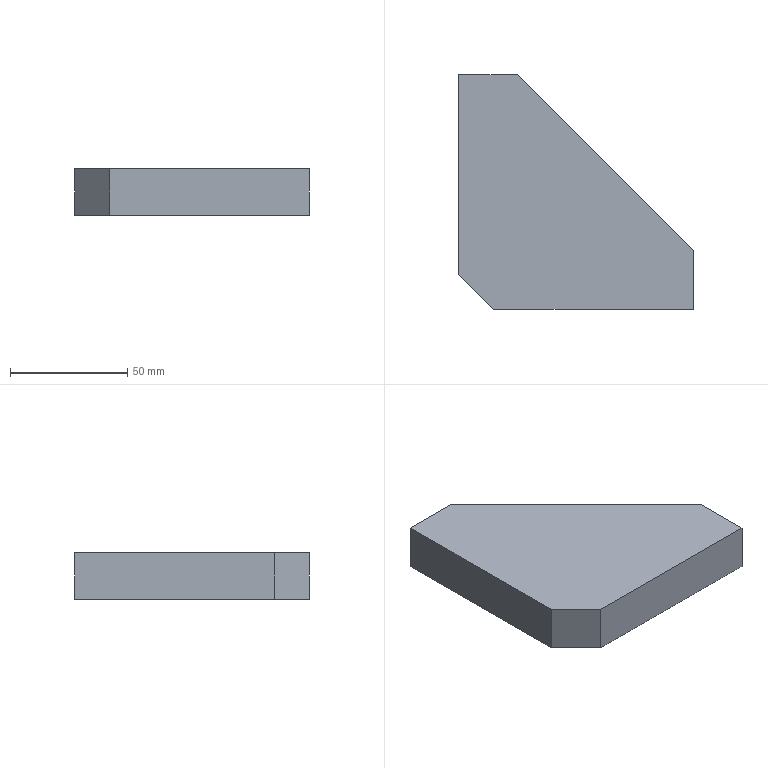Part | SolidWorks | features Chamfer 1, Extrusion 1 | 1 solid | 8 faces | box 100 x 100 x 20 mm | volume 141500 mm3 | plane 8
STEP:
#1=CARTESIAN_POINT('',(0.,100.,0.));
#2=VERTEX_POINT('',#1);
#3=CARTESIAN_POINT('',(0.,15.,0.));
#4=VERTEX_POINT('',#3);
#5=CARTESIAN_POINT('',(0.,100.,0.));
#6=DIRECTION('',(0.,-1.,0.));
#7=VECTOR('',#6,1000.);
#8=LINE('',#5,#7);
#9=EDGE_CURVE('',#2,#4,#8,.T.);
#10=ORIENTED_EDGE('',*,*,#9,.T.);
#11=CARTESIAN_POINT('',(0.,15.,20.));
#12=VERTEX_POINT('',#11);
#13=CARTESIAN_POINT('',(0.,15.,20.));
#14=DIRECTION('',(0.,0.,1.));
#15=VECTOR('',#14,1000.);
#16=LINE('',#13,#15);
#17=EDGE_CURVE('',#4,#12,#16,.T.);
#18=ORIENTED_EDGE('',*,*,#17,.T.);
#19=CARTESIAN_POINT('',(0.,100.,20.));
#20=VERTEX_POINT('',#19);
#21=CARTESIAN_POINT('',(0.,100.,20.));
#22=DIRECTION('',(0.,-1.,0.));
#23=VECTOR('',#22,1000.);
#24=LINE('',#21,#23);
#25=EDGE_CURVE('',#20,#12,#24,.T.);
#26=ORIENTED_EDGE('',*,*,#25,.F.);
#27=CARTESIAN_POINT('',(0.,100.,20.));
#28=DIRECTION('',(0.,0.,-1.));
#29=VECTOR('',#28,1000.);
#30=LINE('',#27,#29);
#31=EDGE_CURVE('',#20,#2,#30,.T.);
#32=ORIENTED_EDGE('',*,*,#31,.T.);
#33=EDGE_LOOP('',(#10,#18,#26,#32));
#34=FACE_OUTER_BOUND('',#33,.T.);
#35=CARTESIAN_POINT('',(0.,100.,20.));
#36=DIRECTION('',(1.,0.,0.));
#37=DIRECTION('',(0.,1.,0.));
#38=AXIS2_PLACEMENT_3D('',#35,#36,#37);
#39=PLANE('',#38);
#40=ADVANCED_FACE('',(#34),#39,.F.);
#41=CARTESIAN_POINT('',(15.,0.,20.));
#42=VERTEX_POINT('',#41);
#43=CARTESIAN_POINT('',(100.,0.,20.));
#44=VERTEX_POINT('',#43);
#45=CARTESIAN_POINT('',(0.,0.,20.));
#46=DIRECTION('',(1.,0.,0.));
#47=VECTOR('',#46,1000.);
#48=LINE('',#45,#47);
#49=EDGE_CURVE('',#42,#44,#48,.T.);
#50=ORIENTED_EDGE('',*,*,#49,.F.);
#51=CARTESIAN_POINT('',(15.,0.,0.));
#52=VERTEX_POINT('',#51);
#53=CARTESIAN_POINT('',(15.,0.,20.));
#54=DIRECTION('',(0.,0.,-1.));
#55=VECTOR('',#54,1000.);
#56=LINE('',#53,#55);
#57=EDGE_CURVE('',#42,#52,#56,.T.);
#58=ORIENTED_EDGE('',*,*,#57,.T.);
#59=CARTESIAN_POINT('',(100.,0.,0.));
#60=VERTEX_POINT('',#59);
#61=CARTESIAN_POINT('',(0.,0.,0.));
#62=DIRECTION('',(1.,0.,0.));
#63=VECTOR('',#62,1000.);
#64=LINE('',#61,#63);
#65=EDGE_CURVE('',#52,#60,#64,.T.);
#66=ORIENTED_EDGE('',*,*,#65,.T.);
#67=CARTESIAN_POINT('',(100.,0.,20.));
#68=DIRECTION('',(0.,0.,-1.));
#69=VECTOR('',#68,1000.);
#70=LINE('',#67,#69);
#71=EDGE_CURVE('',#44,#60,#70,.T.);
#72=ORIENTED_EDGE('',*,*,#71,.F.);
#73=EDGE_LOOP('',(#50,#58,#66,#72));
#74=FACE_OUTER_BOUND('',#73,.T.);
#75=CARTESIAN_POINT('',(0.,0.,20.));
#76=DIRECTION('',(0.,1.,0.));
#77=DIRECTION('',(0.,0.,1.));
#78=AXIS2_PLACEMENT_3D('',#75,#76,#77);
#79=PLANE('',#78);
#80=ADVANCED_FACE('',(#74),#79,.F.);
#81=CARTESIAN_POINT('',(100.,25.,0.));
#82=VERTEX_POINT('',#81);
#83=CARTESIAN_POINT('',(100.,0.,0.));
#84=DIRECTION('',(0.,1.,0.));
#85=VECTOR('',#84,1000.);
#86=LINE('',#83,#85);
#87=EDGE_CURVE('',#60,#82,#86,.T.);
#88=ORIENTED_EDGE('',*,*,#87,.T.);
#89=CARTESIAN_POINT('',(100.,25.,20.));
#90=VERTEX_POINT('',#89);
#91=CARTESIAN_POINT('',(100.,25.,20.));
#92=DIRECTION('',(0.,0.,-1.));
#93=VECTOR('',#92,1000.);
#94=LINE('',#91,#93);
#95=EDGE_CURVE('',#90,#82,#94,.T.);
#96=ORIENTED_EDGE('',*,*,#95,.F.);
#97=CARTESIAN_POINT('',(100.,0.,20.));
#98=DIRECTION('',(0.,1.,0.));
#99=VECTOR('',#98,1000.);
#100=LINE('',#97,#99);
#101=EDGE_CURVE('',#44,#90,#100,.T.);
#102=ORIENTED_EDGE('',*,*,#101,.F.);
#103=ORIENTED_EDGE('',*,*,#71,.T.);
#104=EDGE_LOOP('',(#88,#96,#102,#103));
#105=FACE_OUTER_BOUND('',#104,.T.);
#106=CARTESIAN_POINT('',(100.,0.,20.));
#107=DIRECTION('',(-1.,0.,0.));
#108=DIRECTION('',(0.,0.,1.));
#109=AXIS2_PLACEMENT_3D('',#106,#107,#108);
#110=PLANE('',#109);
#111=ADVANCED_FACE('',(#105),#110,.F.);
#112=CARTESIAN_POINT('',(25.,100.,0.));
#113=VERTEX_POINT('',#112);
#114=CARTESIAN_POINT('',(100.,25.,0.));
#115=DIRECTION('',(-0.7071,0.7071,0.));
#116=VECTOR('',#115,1000.);
#117=LINE('',#114,#116);
#118=EDGE_CURVE('',#82,#113,#117,.T.);
#119=ORIENTED_EDGE('',*,*,#118,.T.);
#120=CARTESIAN_POINT('',(25.,100.,20.));
#121=VERTEX_POINT('',#120);
#122=CARTESIAN_POINT('',(25.,100.,20.));
#123=DIRECTION('',(0.,0.,-1.));
#124=VECTOR('',#123,1000.);
#125=LINE('',#122,#124);
#126=EDGE_CURVE('',#121,#113,#125,.T.);
#127=ORIENTED_EDGE('',*,*,#126,.F.);
#128=CARTESIAN_POINT('',(100.,25.,20.));
#129=DIRECTION('',(-0.7071,0.7071,0.));
#130=VECTOR('',#129,1000.);
#131=LINE('',#128,#130);
#132=EDGE_CURVE('',#90,#121,#131,.T.);
#133=ORIENTED_EDGE('',*,*,#132,.F.);
#134=ORIENTED_EDGE('',*,*,#95,.T.);
#135=EDGE_LOOP('',(#119,#127,#133,#134));
#136=FACE_OUTER_BOUND('',#135,.T.);
#137=CARTESIAN_POINT('',(100.,25.,20.));
#138=DIRECTION('',(-0.7071,-0.7071,0.));
#139=DIRECTION('',(0.7071,-0.7071,0.));
#140=AXIS2_PLACEMENT_3D('',#137,#138,#139);
#141=PLANE('',#140);
#142=ADVANCED_FACE('',(#136),#141,.F.);
#143=CARTESIAN_POINT('',(25.,100.,0.));
#144=DIRECTION('',(-1.,0.,0.));
#145=VECTOR('',#144,1000.);
#146=LINE('',#143,#145);
#147=EDGE_CURVE('',#113,#2,#146,.T.);
#148=ORIENTED_EDGE('',*,*,#147,.T.);
#149=ORIENTED_EDGE('',*,*,#31,.F.);
#150=CARTESIAN_POINT('',(25.,100.,20.));
#151=DIRECTION('',(-1.,0.,0.));
#152=VECTOR('',#151,1000.);
#153=LINE('',#150,#152);
#154=EDGE_CURVE('',#121,#20,#153,.T.);
#155=ORIENTED_EDGE('',*,*,#154,.F.);
#156=ORIENTED_EDGE('',*,*,#126,.T.);
#157=EDGE_LOOP('',(#148,#149,#155,#156));
#158=FACE_OUTER_BOUND('',#157,.T.);
#159=CARTESIAN_POINT('',(25.,100.,20.));
#160=DIRECTION('',(0.,-1.,0.));
#161=DIRECTION('',(0.,0.,-1.));
#162=AXIS2_PLACEMENT_3D('',#159,#160,#161);
#163=PLANE('',#162);
#164=ADVANCED_FACE('',(#158),#163,.F.);
#165=ORIENTED_EDGE('',*,*,#25,.T.);
#166=CARTESIAN_POINT('',(7.5,7.5,20.));
#167=DIRECTION('',(0.7071,-0.7071,0.));
#168=VECTOR('',#167,1000.);
#169=LINE('',#166,#168);
#170=EDGE_CURVE('',#12,#42,#169,.T.);
#171=ORIENTED_EDGE('',*,*,#170,.T.);
#172=ORIENTED_EDGE('',*,*,#49,.T.);
#173=ORIENTED_EDGE('',*,*,#101,.T.);
#174=ORIENTED_EDGE('',*,*,#132,.T.);
#175=ORIENTED_EDGE('',*,*,#154,.T.);
#176=EDGE_LOOP('',(#165,#171,#172,#173,#174,#175));
#177=FACE_OUTER_BOUND('',#176,.T.);
#178=CARTESIAN_POINT('',(0.,0.,20.));
#179=DIRECTION('',(0.,0.,1.));
#180=DIRECTION('',(1.,0.,0.));
#181=AXIS2_PLACEMENT_3D('',#178,#179,#180);
#182=PLANE('',#181);
#183=ADVANCED_FACE('',(#177),#182,.T.);
#184=ORIENTED_EDGE('',*,*,#65,.F.);
#185=CARTESIAN_POINT('',(15.,0.,0.));
#186=DIRECTION('',(-0.7071,0.7071,0.));
#187=VECTOR('',#186,1000.);
#188=LINE('',#185,#187);
#189=EDGE_CURVE('',#52,#4,#188,.T.);
#190=ORIENTED_EDGE('',*,*,#189,.T.);
#191=ORIENTED_EDGE('',*,*,#9,.F.);
#192=ORIENTED_EDGE('',*,*,#147,.F.);
#193=ORIENTED_EDGE('',*,*,#118,.F.);
#194=ORIENTED_EDGE('',*,*,#87,.F.);
#195=EDGE_LOOP('',(#184,#190,#191,#192,#193,#194));
#196=FACE_OUTER_BOUND('',#195,.T.);
#197=CARTESIAN_POINT('',(0.,0.,0.));
#198=DIRECTION('',(0.,0.,1.));
#199=DIRECTION('',(1.,0.,0.));
#200=AXIS2_PLACEMENT_3D('',#197,#198,#199);
#201=PLANE('',#200);
#202=ADVANCED_FACE('',(#196),#201,.F.);
#203=ORIENTED_EDGE('',*,*,#170,.F.);
#204=ORIENTED_EDGE('',*,*,#17,.F.);
#205=ORIENTED_EDGE('',*,*,#189,.F.);
#206=ORIENTED_EDGE('',*,*,#57,.F.);
#207=EDGE_LOOP('',(#203,#204,#205,#206));
#208=FACE_OUTER_BOUND('',#207,.T.);
#209=CARTESIAN_POINT('',(15.,0.,20.));
#210=DIRECTION('',(0.7071,0.7071,0.));
#211=DIRECTION('',(0.,0.,-1.));
#212=AXIS2_PLACEMENT_3D('',#209,#210,#211);
#213=PLANE('',#212);
#214=ADVANCED_FACE('',(#208),#213,.F.);
#215=CLOSED_SHELL('',(#40,#80,#111,#142,#164,#183,#202,#214));
#216=MANIFOLD_SOLID_BREP('',#215);
#217=CARTESIAN_POINT('',(0.,0.,0.));
#218=DIRECTION('',(0.,0.,1.));
#219=DIRECTION('',(1.,0.,0.));
#220=AXIS2_PLACEMENT_3D('',#217,#218,#219);
#221=(LENGTH_UNIT()NAMED_UNIT(*)SI_UNIT(.MILLI.,.METRE.));
#222=UNCERTAINTY_MEASURE_WITH_UNIT(LENGTH_MEASURE(0.00001),#221,'','');
#223=(NAMED_UNIT(*)PLANE_ANGLE_UNIT()SI_UNIT($,.RADIAN.));
#224=(NAMED_UNIT(*)SI_UNIT($,.STERADIAN.)SOLID_ANGLE_UNIT());
#225=(GEOMETRIC_REPRESENTATION_CONTEXT(3)GLOBAL_UNCERTAINTY_ASSIGNED_CONTEXT((#222))GLOBAL_UNIT_ASSIGNED_CONTEXT((#221,#223,#224))REPRESENTATION_CONTEXT('',''));
#226=ADVANCED_BREP_SHAPE_REPRESENTATION('',(#216,#220),#225);